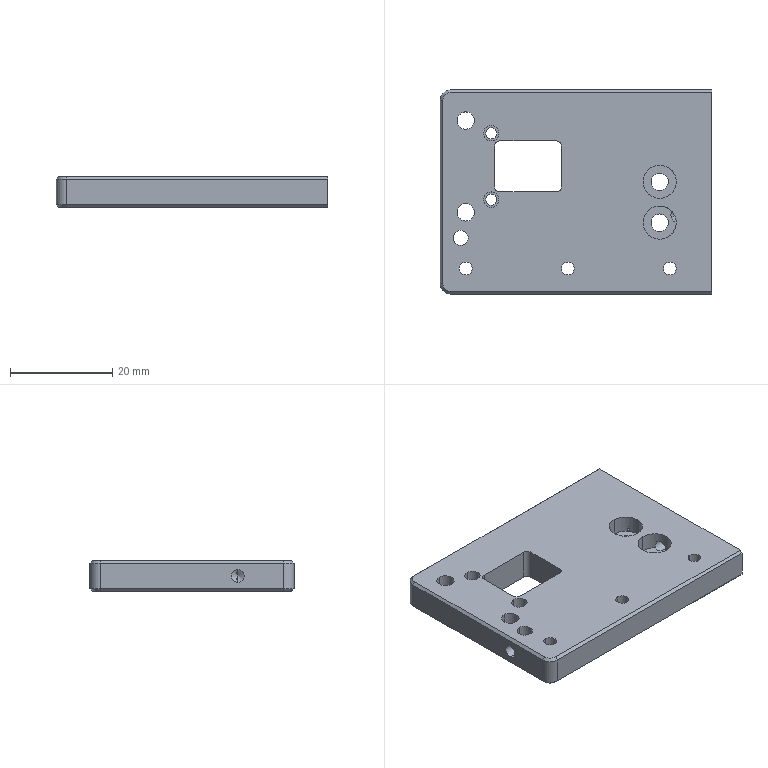Part | 1 solid | 93 faces | box 53.2 x 40 x 6 mm | volume 10963 mm3 | cylinder 52 | plane 26 | cone 15 | commonest cylinder face diameters 2.5 x16 3 x10 3.4 x8 6.5 x8 2 x4 2.2 x4